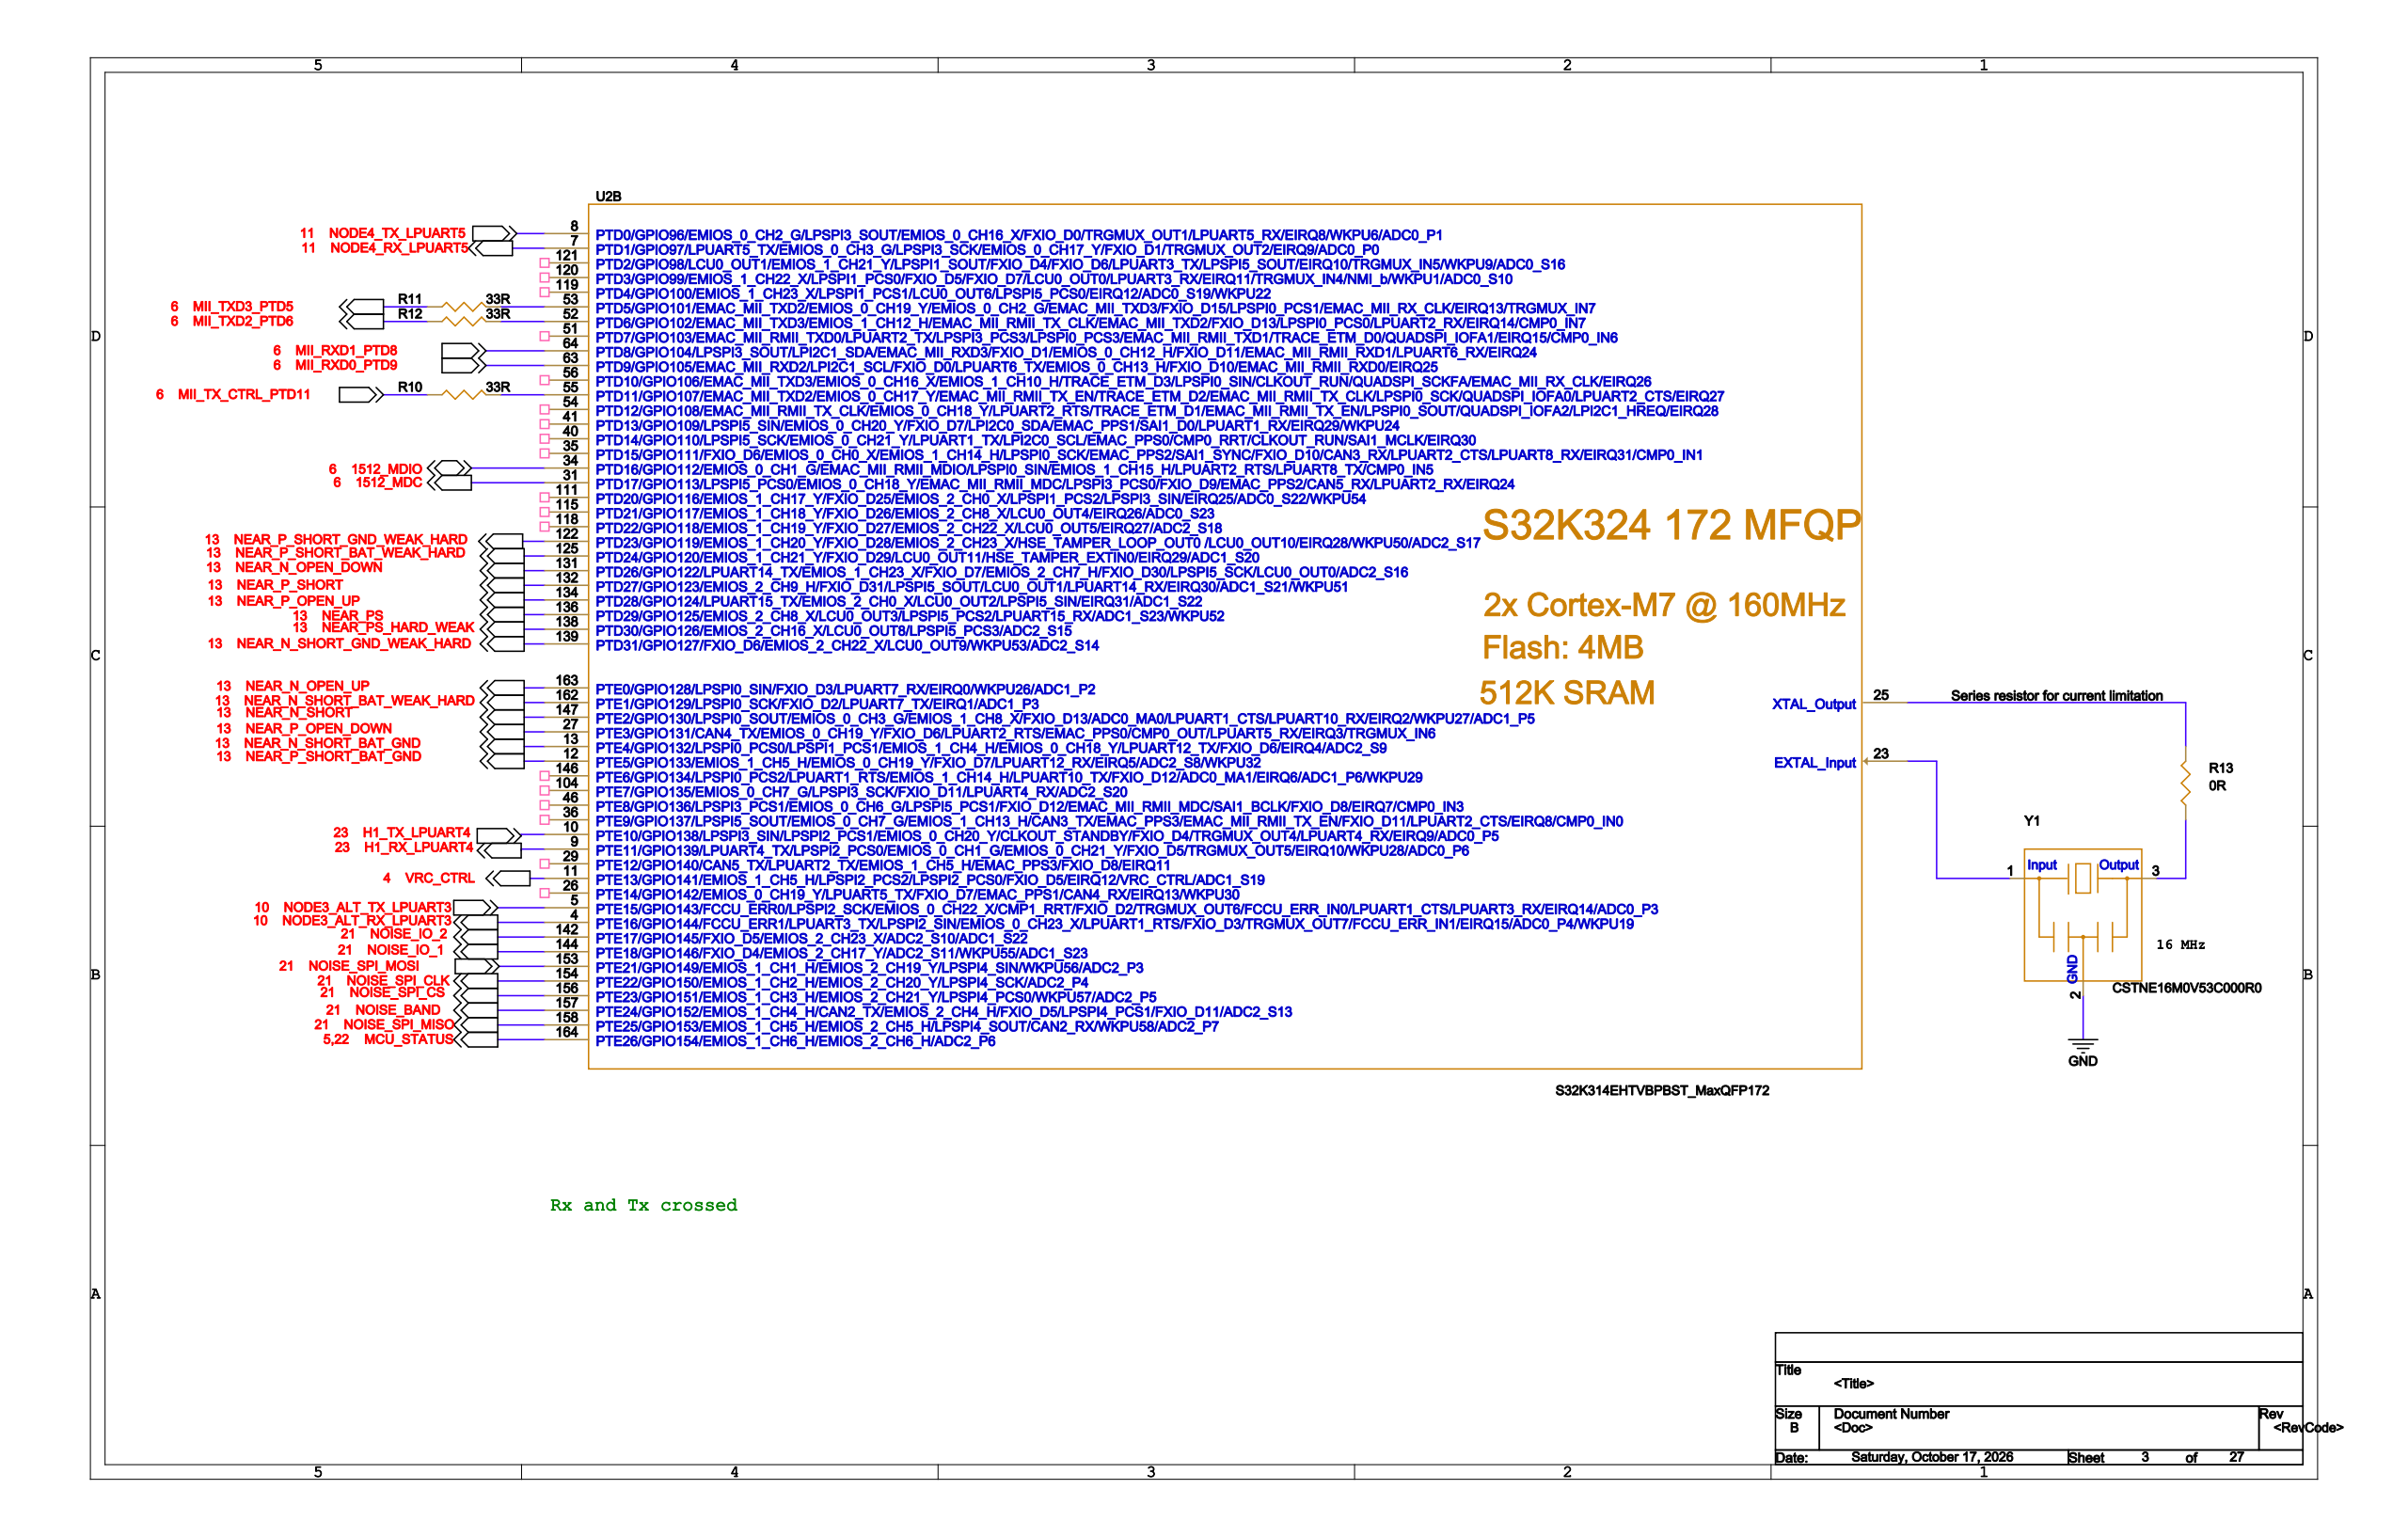Circuit board | Cadence Allegro | 477 parts | 327 nets | one sheet of the schematic
Parts on this sheet (reference | value | footprint):
R10 | 33R | 0402
R11 | 33R | 0402
R12 | 33R | 0402
R13 | 0R | 0402
U2 | S32K314EHTVBPBST_MaxQFP172 | MQFP172_0P65_16X16
Y1 | CSTNE16M0V53C000R0 | CSTNE16M0V53C000R0
Nets of these parts (net: part-pin ...):
MII_TX_CTRL_PTD11: R10-1
N2514195: R10-2 U2-55
MII_TXD3_PTD5: R11-1
N2514215: R11-2 U2-53
MII_TXD2_PTD6: R12-1
N2514203: R12-2 U2-52
MII_RXD0_PTD9: U2-63
MII_RXD1_PTD8: U2-64
NEAR_P_OPEN_DOWN: U2-27
NEAR_P_SHORT_BAT_WEAK_HARD: U2-125
NEAR_N_SHORT_BAT_WEAK_HARD: U2-162
NEAR_P_SHORT_BAT_GND: U2-12
NEAR_P_SHORT: U2-132
NEAR_N_SHORT: U2-147
NEAR_N_SHORT_BAT_GND: U2-13
NEAR_PS_HARD_WEAK: U2-138
NEAR_P_SHORT_GND_WEAK_HARD: U2-122
NEAR_N_SHORT_GND_WEAK_HARD: U2-139
NEAR_PS: U2-136
NEAR_P_OPEN_UP: U2-134
NEAR_N_OPEN_UP: U2-163
NEAR_N_OPEN_DOWN: U2-131
GND: Y1-2 U2-17 U2-22
1512_MDC: U2-31
1512_MDIO: U2-34
N1671028: R13-1 Y1-3
N1670986: R13-2 U2-25
VRC_CTRL: U2-11
NOISE_SPI_CS: U2-156
NOISE_IO_1: U2-144
MCU_STATUS: U2-164
NOISE_SPI_MISO: U2-158
NOISE_SPI_CLK: U2-154
NOISE_BAND: U2-157
NOISE_IO_2: U2-142
NOISE_SPI_MOSI: U2-153
H1_TX_LPUART4: U2-10
H1_RX_LPUART4: U2-9
NODE3_ALT_TX_LPUART3: U2-5
NODE3_ALT_RX_LPUART3: U2-4
NODE4_TX_LPUART5: U2-8
NODE4_RX_LPUART5: U2-7
N1670994: Y1-1 U2-23